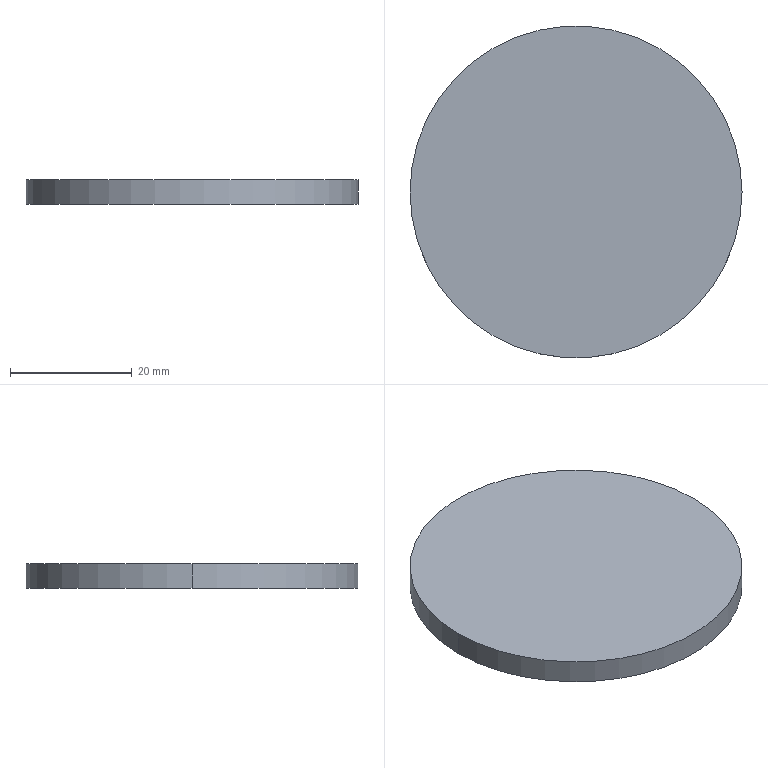Part | SolidWorks | features Extrusion 1 | 1 solid | 4 faces | box 54.5 x 54.5 x 4 mm | volume 9331 mm3 | cylinder 2 | plane 2 | commonest cylinder face diameters 54.5 x2
STEP:
#1=CARTESIAN_POINT('',(27.25,0.,4.));
#2=VERTEX_POINT('',#1);
#3=CARTESIAN_POINT('',(-27.25,0.,4.));
#4=VERTEX_POINT('',#3);
#5=CARTESIAN_POINT('',(0.,0.,4.));
#6=DIRECTION('',(0.,0.,1.));
#7=DIRECTION('',(1.,0.,0.));
#8=AXIS2_PLACEMENT_3D('',#5,#6,#7);
#9=CIRCLE('',#8,27.25);
#10=EDGE_CURVE('',#2,#4,#9,.T.);
#11=ORIENTED_EDGE('',*,*,#10,.F.);
#12=CARTESIAN_POINT('',(27.25,0.,0.));
#13=VERTEX_POINT('',#12);
#14=CARTESIAN_POINT('',(27.25,0.,4.));
#15=DIRECTION('',(0.,0.,-1.));
#16=VECTOR('',#15,1000.);
#17=LINE('',#14,#16);
#18=EDGE_CURVE('',#2,#13,#17,.T.);
#19=ORIENTED_EDGE('',*,*,#18,.T.);
#20=CARTESIAN_POINT('',(-27.25,0.,0.));
#21=VERTEX_POINT('',#20);
#22=CARTESIAN_POINT('',(0.,0.,0.));
#23=DIRECTION('',(0.,0.,1.));
#24=DIRECTION('',(1.,0.,0.));
#25=AXIS2_PLACEMENT_3D('',#22,#23,#24);
#26=CIRCLE('',#25,27.25);
#27=EDGE_CURVE('',#13,#21,#26,.T.);
#28=ORIENTED_EDGE('',*,*,#27,.T.);
#29=CARTESIAN_POINT('',(-27.25,0.,4.));
#30=DIRECTION('',(0.,0.,-1.));
#31=VECTOR('',#30,1000.);
#32=LINE('',#29,#31);
#33=EDGE_CURVE('',#4,#21,#32,.T.);
#34=ORIENTED_EDGE('',*,*,#33,.F.);
#35=EDGE_LOOP('',(#11,#19,#28,#34));
#36=FACE_OUTER_BOUND('',#35,.T.);
#37=CARTESIAN_POINT('',(0.,0.,4.));
#38=DIRECTION('',(0.,0.,-1.));
#39=DIRECTION('',(-1.,0.,0.));
#40=AXIS2_PLACEMENT_3D('',#37,#38,#39);
#41=CYLINDRICAL_SURFACE('',#40,27.25);
#42=ADVANCED_FACE('',(#36),#41,.T.);
#43=ORIENTED_EDGE('',*,*,#18,.F.);
#44=CARTESIAN_POINT('',(0.,0.,4.));
#45=DIRECTION('',(0.,0.,1.));
#46=DIRECTION('',(1.,0.,0.));
#47=AXIS2_PLACEMENT_3D('',#44,#45,#46);
#48=CIRCLE('',#47,27.25);
#49=EDGE_CURVE('',#4,#2,#48,.T.);
#50=ORIENTED_EDGE('',*,*,#49,.F.);
#51=ORIENTED_EDGE('',*,*,#33,.T.);
#52=CARTESIAN_POINT('',(0.,0.,0.));
#53=DIRECTION('',(0.,0.,1.));
#54=DIRECTION('',(1.,0.,0.));
#55=AXIS2_PLACEMENT_3D('',#52,#53,#54);
#56=CIRCLE('',#55,27.25);
#57=EDGE_CURVE('',#21,#13,#56,.T.);
#58=ORIENTED_EDGE('',*,*,#57,.T.);
#59=EDGE_LOOP('',(#43,#50,#51,#58));
#60=FACE_OUTER_BOUND('',#59,.T.);
#61=CARTESIAN_POINT('',(0.,0.,4.));
#62=DIRECTION('',(0.,0.,-1.));
#63=DIRECTION('',(-1.,0.,0.));
#64=AXIS2_PLACEMENT_3D('',#61,#62,#63);
#65=CYLINDRICAL_SURFACE('',#64,27.25);
#66=ADVANCED_FACE('',(#60),#65,.T.);
#67=ORIENTED_EDGE('',*,*,#49,.T.);
#68=ORIENTED_EDGE('',*,*,#10,.T.);
#69=EDGE_LOOP('',(#67,#68));
#70=FACE_OUTER_BOUND('',#69,.T.);
#71=CARTESIAN_POINT('',(0.,0.,4.));
#72=DIRECTION('',(0.,0.,1.));
#73=DIRECTION('',(1.,0.,0.));
#74=AXIS2_PLACEMENT_3D('',#71,#72,#73);
#75=PLANE('',#74);
#76=ADVANCED_FACE('',(#70),#75,.T.);
#77=ORIENTED_EDGE('',*,*,#57,.F.);
#78=ORIENTED_EDGE('',*,*,#27,.F.);
#79=EDGE_LOOP('',(#77,#78));
#80=FACE_OUTER_BOUND('',#79,.T.);
#81=CARTESIAN_POINT('',(0.,0.,0.));
#82=DIRECTION('',(0.,0.,1.));
#83=DIRECTION('',(1.,0.,0.));
#84=AXIS2_PLACEMENT_3D('',#81,#82,#83);
#85=PLANE('',#84);
#86=ADVANCED_FACE('',(#80),#85,.F.);
#87=CLOSED_SHELL('',(#42,#66,#76,#86));
#88=MANIFOLD_SOLID_BREP('',#87);
#89=CARTESIAN_POINT('',(0.,0.,0.));
#90=DIRECTION('',(0.,0.,1.));
#91=DIRECTION('',(1.,0.,0.));
#92=AXIS2_PLACEMENT_3D('',#89,#90,#91);
#93=(LENGTH_UNIT()NAMED_UNIT(*)SI_UNIT(.MILLI.,.METRE.));
#94=UNCERTAINTY_MEASURE_WITH_UNIT(LENGTH_MEASURE(0.00001),#93,'','');
#95=(NAMED_UNIT(*)PLANE_ANGLE_UNIT()SI_UNIT($,.RADIAN.));
#96=(NAMED_UNIT(*)SI_UNIT($,.STERADIAN.)SOLID_ANGLE_UNIT());
#97=(GEOMETRIC_REPRESENTATION_CONTEXT(3)GLOBAL_UNCERTAINTY_ASSIGNED_CONTEXT((#94))GLOBAL_UNIT_ASSIGNED_CONTEXT((#93,#95,#96))REPRESENTATION_CONTEXT('',''));
#98=ADVANCED_BREP_SHAPE_REPRESENTATION('',(#88,#92),#97);